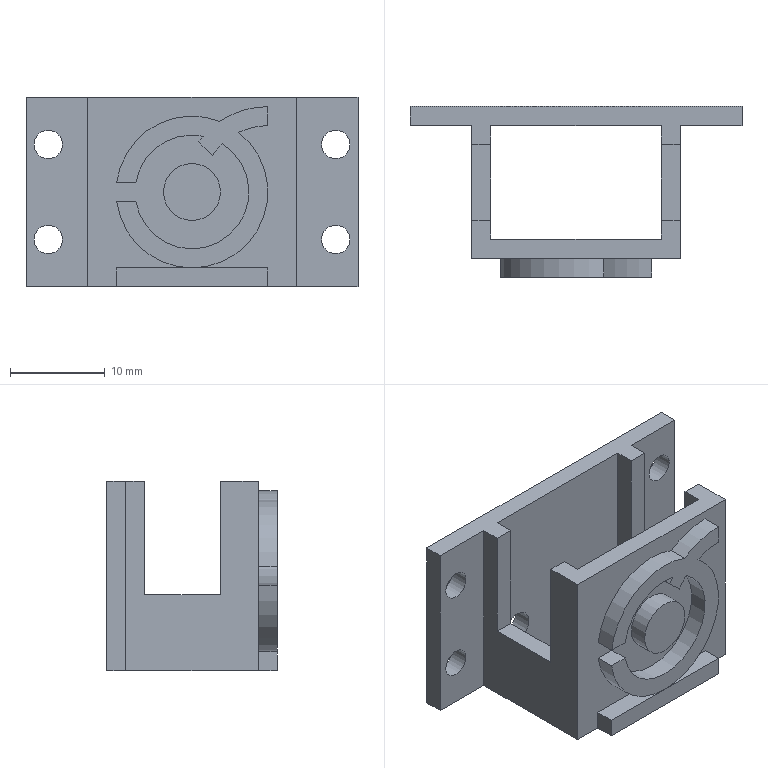Part | NX | features BREP 4 | 4 solids | 50 faces | box 35 x 18 x 20 mm | volume 3071 mm3 | plane 35 | cylinder 15 | commonest cylinder face diameters 3 x4 3.5 x2 12 x2 14 x2 16 x2 18 x2
STEP:
#1=CARTESIAN_POINT('',(-8.,-8.,-10.));
#2=VERTEX_POINT('',#1);
#3=CARTESIAN_POINT('',(-8.,-8.,-8.));
#4=VERTEX_POINT('',#3);
#5=CARTESIAN_POINT('',(-8.,-8.,-8.));
#6=DIRECTION('',(0.,0.,1.));
#7=VECTOR('',#6,1000.);
#8=LINE('',#5,#7);
#9=EDGE_CURVE('',#2,#4,#8,.T.);
#10=ORIENTED_EDGE('',*,*,#9,.F.);
#11=CARTESIAN_POINT('',(-8.,-10.,-10.));
#12=VERTEX_POINT('',#11);
#13=CARTESIAN_POINT('',(-8.,8.125,-10.));
#14=DIRECTION('',(0.,-1.,0.));
#15=VECTOR('',#14,1000.);
#16=LINE('',#13,#15);
#17=EDGE_CURVE('',#2,#12,#16,.T.);
#18=ORIENTED_EDGE('',*,*,#17,.T.);
#19=CARTESIAN_POINT('',(-8.,-10.,-8.));
#20=VERTEX_POINT('',#19);
#21=CARTESIAN_POINT('',(-8.,-10.,-8.));
#22=DIRECTION('',(0.,0.,-1.));
#23=VECTOR('',#22,1000.);
#24=LINE('',#21,#23);
#25=EDGE_CURVE('',#20,#12,#24,.T.);
#26=ORIENTED_EDGE('',*,*,#25,.F.);
#27=CARTESIAN_POINT('',(-8.,8.125,-8.));
#28=DIRECTION('',(0.,-1.,0.));
#29=VECTOR('',#28,1000.);
#30=LINE('',#27,#29);
#31=EDGE_CURVE('',#4,#20,#30,.T.);
#32=ORIENTED_EDGE('',*,*,#31,.F.);
#33=EDGE_LOOP('',(#10,#18,#26,#32));
#34=FACE_BOUND('',#33,.T.);
#35=CARTESIAN_POINT('',(-8.,8.125,-8.));
#36=DIRECTION('',(-1.,0.,0.));
#37=DIRECTION('',(0.,0.,1.));
#38=AXIS2_PLACEMENT_3D('',#35,#36,#37);
#39=PLANE('',#38);
#40=ADVANCED_FACE('',(#34),#39,.T.);
#41=CARTESIAN_POINT('',(8.,-8.,-8.));
#42=VERTEX_POINT('',#41);
#43=CARTESIAN_POINT('',(-8.,-8.,-8.));
#44=DIRECTION('',(1.,0.,0.));
#45=VECTOR('',#44,1000.);
#46=LINE('',#43,#45);
#47=EDGE_CURVE('',#4,#42,#46,.T.);
#48=ORIENTED_EDGE('',*,*,#47,.F.);
#49=ORIENTED_EDGE('',*,*,#31,.T.);
#50=CARTESIAN_POINT('',(8.,-10.,-8.));
#51=VERTEX_POINT('',#50);
#52=CARTESIAN_POINT('',(-8.,-10.,-8.));
#53=DIRECTION('',(-1.,0.,0.));
#54=VECTOR('',#53,1000.);
#55=LINE('',#52,#54);
#56=EDGE_CURVE('',#51,#20,#55,.T.);
#57=ORIENTED_EDGE('',*,*,#56,.F.);
#58=CARTESIAN_POINT('',(8.,8.125,-8.));
#59=DIRECTION('',(0.,-1.,0.));
#60=VECTOR('',#59,1000.);
#61=LINE('',#58,#60);
#62=EDGE_CURVE('',#42,#51,#61,.T.);
#63=ORIENTED_EDGE('',*,*,#62,.F.);
#64=EDGE_LOOP('',(#48,#49,#57,#63));
#65=FACE_BOUND('',#64,.T.);
#66=CARTESIAN_POINT('',(-8.,8.125,-8.));
#67=DIRECTION('',(0.,0.,1.));
#68=DIRECTION('',(1.,0.,0.));
#69=AXIS2_PLACEMENT_3D('',#66,#67,#68);
#70=PLANE('',#69);
#71=ADVANCED_FACE('',(#65),#70,.T.);
#72=CARTESIAN_POINT('',(8.,-8.,-10.));
#73=VERTEX_POINT('',#72);
#74=CARTESIAN_POINT('',(8.,-8.,-8.));
#75=DIRECTION('',(0.,0.,-1.));
#76=VECTOR('',#75,1000.);
#77=LINE('',#74,#76);
#78=EDGE_CURVE('',#42,#73,#77,.T.);
#79=ORIENTED_EDGE('',*,*,#78,.F.);
#80=ORIENTED_EDGE('',*,*,#62,.T.);
#81=CARTESIAN_POINT('',(8.,-10.,-10.));
#82=VERTEX_POINT('',#81);
#83=CARTESIAN_POINT('',(8.,-10.,-8.));
#84=DIRECTION('',(0.,0.,1.));
#85=VECTOR('',#84,1000.);
#86=LINE('',#83,#85);
#87=EDGE_CURVE('',#82,#51,#86,.T.);
#88=ORIENTED_EDGE('',*,*,#87,.F.);
#89=CARTESIAN_POINT('',(8.,8.125,-10.));
#90=DIRECTION('',(0.,-1.,0.));
#91=VECTOR('',#90,1000.);
#92=LINE('',#89,#91);
#93=EDGE_CURVE('',#73,#82,#92,.T.);
#94=ORIENTED_EDGE('',*,*,#93,.F.);
#95=EDGE_LOOP('',(#79,#80,#88,#94));
#96=FACE_BOUND('',#95,.T.);
#97=CARTESIAN_POINT('',(8.,8.125,-8.));
#98=DIRECTION('',(1.,0.,0.));
#99=DIRECTION('',(0.,-1.,0.));
#100=AXIS2_PLACEMENT_3D('',#97,#98,#99);
#101=PLANE('',#100);
#102=ADVANCED_FACE('',(#96),#101,.T.);
#103=CARTESIAN_POINT('',(-8.,-8.,-10.));
#104=DIRECTION('',(-1.,0.,0.));
#105=VECTOR('',#104,1000.);
#106=LINE('',#103,#105);
#107=EDGE_CURVE('',#73,#2,#106,.T.);
#108=ORIENTED_EDGE('',*,*,#107,.F.);
#109=ORIENTED_EDGE('',*,*,#93,.T.);
#110=CARTESIAN_POINT('',(-8.,-10.,-10.));
#111=DIRECTION('',(1.,0.,0.));
#112=VECTOR('',#111,1000.);
#113=LINE('',#110,#112);
#114=EDGE_CURVE('',#12,#82,#113,.T.);
#115=ORIENTED_EDGE('',*,*,#114,.F.);
#116=ORIENTED_EDGE('',*,*,#17,.F.);
#117=EDGE_LOOP('',(#108,#109,#115,#116));
#118=FACE_BOUND('',#117,.T.);
#119=CARTESIAN_POINT('',(-8.,8.125,-10.));
#120=DIRECTION('',(0.,0.,-1.));
#121=DIRECTION('',(-1.,0.,0.));
#122=AXIS2_PLACEMENT_3D('',#119,#120,#121);
#123=PLANE('',#122);
#124=ADVANCED_FACE('',(#118),#123,.T.);
#125=ORIENTED_EDGE('',*,*,#25,.T.);
#126=ORIENTED_EDGE('',*,*,#114,.T.);
#127=ORIENTED_EDGE('',*,*,#87,.T.);
#128=ORIENTED_EDGE('',*,*,#56,.T.);
#129=EDGE_LOOP('',(#125,#126,#127,#128));
#130=FACE_BOUND('',#129,.T.);
#131=CARTESIAN_POINT('',(0.,-10.,0.));
#132=DIRECTION('',(0.,-1.,0.));
#133=DIRECTION('',(-1.,0.,0.));
#134=AXIS2_PLACEMENT_3D('',#131,#132,#133);
#135=PLANE('',#134);
#136=ADVANCED_FACE('',(#130),#135,.T.);
#137=ORIENTED_EDGE('',*,*,#9,.T.);
#138=ORIENTED_EDGE('',*,*,#47,.T.);
#139=ORIENTED_EDGE('',*,*,#78,.T.);
#140=ORIENTED_EDGE('',*,*,#107,.T.);
#141=EDGE_LOOP('',(#137,#138,#139,#140));
#142=FACE_BOUND('',#141,.T.);
#143=CARTESIAN_POINT('',(0.,-8.,0.));
#144=DIRECTION('',(0.,-1.,0.));
#145=DIRECTION('',(-1.,0.,0.));
#146=AXIS2_PLACEMENT_3D('',#143,#144,#145);
#147=PLANE('',#146);
#148=ADVANCED_FACE('',(#142),#147,.F.);
#149=CLOSED_SHELL('',(#40,#71,#102,#124,#136,#148));
#150=MANIFOLD_SOLID_BREP('',#149);
#151=CARTESIAN_POINT('',(3.,-10.,0.));
#152=VERTEX_POINT('',#151);
#153=CARTESIAN_POINT('',(0.,-10.,0.));
#154=DIRECTION('',(0.,-1.,0.));
#155=DIRECTION('',(1.,0.,0.));
#156=AXIS2_PLACEMENT_3D('',#153,#154,#155);
#157=CIRCLE('',#156,3.);
#158=EDGE_CURVE('',#152,#152,#157,.T.);
#159=ORIENTED_EDGE('',*,*,#158,.F.);
#160=EDGE_LOOP('',(#159));
#161=FACE_BOUND('',#160,.T.);
#162=CARTESIAN_POINT('',(3.,-8.,0.));
#163=VERTEX_POINT('',#162);
#164=CARTESIAN_POINT('',(0.,-8.,0.));
#165=DIRECTION('',(0.,1.,0.));
#166=DIRECTION('',(1.,0.,0.));
#167=AXIS2_PLACEMENT_3D('',#164,#165,#166);
#168=CIRCLE('',#167,3.);
#169=EDGE_CURVE('',#163,#163,#168,.T.);
#170=ORIENTED_EDGE('',*,*,#169,.F.);
#171=EDGE_LOOP('',(#170));
#172=FACE_BOUND('',#171,.T.);
#173=CARTESIAN_POINT('',(0.,0.4853,0.));
#174=DIRECTION('',(0.,-1.,0.));
#175=DIRECTION('',(-1.,0.,0.));
#176=AXIS2_PLACEMENT_3D('',#173,#174,#175);
#177=CYLINDRICAL_SURFACE('',#176,3.);
#178=ADVANCED_FACE('',(#161,#172),#177,.T.);
#179=ORIENTED_EDGE('',*,*,#158,.T.);
#180=EDGE_LOOP('',(#179));
#181=FACE_BOUND('',#180,.T.);
#182=CARTESIAN_POINT('',(0.,-10.,0.));
#183=DIRECTION('',(0.,-1.,0.));
#184=DIRECTION('',(-1.,0.,0.));
#185=AXIS2_PLACEMENT_3D('',#182,#183,#184);
#186=PLANE('',#185);
#187=ADVANCED_FACE('',(#181),#186,.T.);
#188=ORIENTED_EDGE('',*,*,#169,.T.);
#189=EDGE_LOOP('',(#188));
#190=FACE_BOUND('',#189,.T.);
#191=CARTESIAN_POINT('',(0.,-8.,0.));
#192=DIRECTION('',(0.,-1.,0.));
#193=DIRECTION('',(-1.,0.,0.));
#194=AXIS2_PLACEMENT_3D('',#191,#192,#193);
#195=PLANE('',#194);
#196=ADVANCED_FACE('',(#190),#195,.F.);
#197=CLOSED_SHELL('',(#178,#187,#196));
#198=MANIFOLD_SOLID_BREP('',#197);
#199=CARTESIAN_POINT('',(2.938,-8.,7.441));
#200=VERTEX_POINT('',#199);
#201=CARTESIAN_POINT('',(-7.937,-8.,1.));
#202=VERTEX_POINT('',#201);
#203=CARTESIAN_POINT('',(0.,-8.,0.));
#204=DIRECTION('',(0.,-1.,0.));
#205=DIRECTION('',(1.,0.,0.));
#206=AXIS2_PLACEMENT_3D('',#203,#204,#205);
#207=CIRCLE('',#206,8.);
#208=EDGE_CURVE('',#200,#202,#207,.T.);
#209=ORIENTED_EDGE('',*,*,#208,.T.);
#210=CARTESIAN_POINT('',(-7.937,-10.,1.));
#211=VERTEX_POINT('',#210);
#212=CARTESIAN_POINT('',(-7.937,-10.,1.));
#213=DIRECTION('',(0.,-1.,0.));
#214=VECTOR('',#213,1000.);
#215=LINE('',#212,#214);
#216=EDGE_CURVE('',#202,#211,#215,.T.);
#217=ORIENTED_EDGE('',*,*,#216,.T.);
#218=CARTESIAN_POINT('',(2.938,-10.,7.441));
#219=VERTEX_POINT('',#218);
#220=CARTESIAN_POINT('',(0.,-10.,0.));
#221=DIRECTION('',(0.,-1.,0.));
#222=DIRECTION('',(1.,0.,0.));
#223=AXIS2_PLACEMENT_3D('',#220,#221,#222);
#224=CIRCLE('',#223,8.);
#225=EDGE_CURVE('',#219,#211,#224,.T.);
#226=ORIENTED_EDGE('',*,*,#225,.F.);
#227=CARTESIAN_POINT('',(2.938,-9.,7.441));
#228=DIRECTION('',(0.,1.,0.));
#229=VECTOR('',#228,1000.);
#230=LINE('',#227,#229);
#231=EDGE_CURVE('',#219,#200,#230,.T.);
#232=ORIENTED_EDGE('',*,*,#231,.T.);
#233=EDGE_LOOP('',(#209,#217,#226,#232));
#234=FACE_BOUND('',#233,.T.);
#235=CARTESIAN_POINT('',(0.,-10.,0.));
#236=DIRECTION('',(0.,1.,0.));
#237=DIRECTION('',(1.,0.,0.));
#238=AXIS2_PLACEMENT_3D('',#235,#236,#237);
#239=CYLINDRICAL_SURFACE('',#238,8.);
#240=ADVANCED_FACE('',(#234),#239,.T.);
#241=CARTESIAN_POINT('',(-5.916,-8.,1.));
#242=VERTEX_POINT('',#241);
#243=CARTESIAN_POINT('',(-5.916,-10.,1.));
#244=VERTEX_POINT('',#243);
#245=CARTESIAN_POINT('',(-5.916,-10.,1.));
#246=DIRECTION('',(0.,-1.,0.));
#247=VECTOR('',#246,1000.);
#248=LINE('',#245,#247);
#249=EDGE_CURVE('',#242,#244,#248,.T.);
#250=ORIENTED_EDGE('',*,*,#249,.F.);
#251=CARTESIAN_POINT('',(1.188,-8.,5.881));
#252=VERTEX_POINT('',#251);
#253=CARTESIAN_POINT('',(0.,-8.,0.));
#254=DIRECTION('',(0.,-1.,0.));
#255=DIRECTION('',(1.,0.,0.));
#256=AXIS2_PLACEMENT_3D('',#253,#254,#255);
#257=CIRCLE('',#256,6.);
#258=EDGE_CURVE('',#252,#242,#257,.T.);
#259=ORIENTED_EDGE('',*,*,#258,.F.);
#260=CARTESIAN_POINT('',(1.188,-10.,5.881));
#261=VERTEX_POINT('',#260);
#262=CARTESIAN_POINT('',(1.188,-9.,5.881));
#263=DIRECTION('',(0.,1.,0.));
#264=VECTOR('',#263,1000.);
#265=LINE('',#262,#264);
#266=EDGE_CURVE('',#261,#252,#265,.T.);
#267=ORIENTED_EDGE('',*,*,#266,.F.);
#268=CARTESIAN_POINT('',(0.,-10.,0.));
#269=DIRECTION('',(0.,-1.,0.));
#270=DIRECTION('',(1.,0.,0.));
#271=AXIS2_PLACEMENT_3D('',#268,#269,#270);
#272=CIRCLE('',#271,6.);
#273=EDGE_CURVE('',#261,#244,#272,.T.);
#274=ORIENTED_EDGE('',*,*,#273,.T.);
#275=EDGE_LOOP('',(#250,#259,#267,#274));
#276=FACE_BOUND('',#275,.T.);
#277=CARTESIAN_POINT('',(0.,-10.,0.));
#278=DIRECTION('',(0.,1.,0.));
#279=DIRECTION('',(1.,0.,0.));
#280=AXIS2_PLACEMENT_3D('',#277,#278,#279);
#281=CYLINDRICAL_SURFACE('',#280,6.);
#282=ADVANCED_FACE('',(#276),#281,.F.);
#283=CARTESIAN_POINT('',(-10.409,-10.,1.));
#284=DIRECTION('',(-1.,0.,0.));
#285=VECTOR('',#284,1000.);
#286=LINE('',#283,#285);
#287=EDGE_CURVE('',#244,#211,#286,.T.);
#288=ORIENTED_EDGE('',*,*,#287,.F.);
#289=ORIENTED_EDGE('',*,*,#273,.F.);
#290=CARTESIAN_POINT('',(0.7151,-10.,5.285));
#291=VERTEX_POINT('',#290);
#292=CARTESIAN_POINT('',(8.,-10.,0.));
#293=DIRECTION('',(0.,-1.,0.));
#294=DIRECTION('',(1.,0.,0.));
#295=AXIS2_PLACEMENT_3D('',#292,#293,#294);
#296=CIRCLE('',#295,9.);
#297=EDGE_CURVE('',#261,#291,#296,.T.);
#298=ORIENTED_EDGE('',*,*,#297,.T.);
#299=CARTESIAN_POINT('',(2.152,-10.,3.848));
#300=VERTEX_POINT('',#299);
#301=CARTESIAN_POINT('',(2.152,-10.,3.848));
#302=DIRECTION('',(0.7071,0.,-0.7071));
#303=VECTOR('',#302,1000.);
#304=LINE('',#301,#303);
#305=EDGE_CURVE('',#291,#300,#304,.T.);
#306=ORIENTED_EDGE('',*,*,#305,.T.);
#307=CARTESIAN_POINT('',(3.188,-10.,5.083));
#308=VERTEX_POINT('',#307);
#309=CARTESIAN_POINT('',(8.,-10.,0.));
#310=DIRECTION('',(0.,1.,0.));
#311=DIRECTION('',(1.,0.,0.));
#312=AXIS2_PLACEMENT_3D('',#309,#310,#311);
#313=CIRCLE('',#312,7.);
#314=EDGE_CURVE('',#300,#308,#313,.T.);
#315=ORIENTED_EDGE('',*,*,#314,.T.);
#316=CARTESIAN_POINT('',(-5.916,-10.,-1.));
#317=VERTEX_POINT('',#316);
#318=CARTESIAN_POINT('',(0.,-10.,0.));
#319=DIRECTION('',(0.,-1.,0.));
#320=DIRECTION('',(1.,0.,0.));
#321=AXIS2_PLACEMENT_3D('',#318,#319,#320);
#322=CIRCLE('',#321,6.);
#323=EDGE_CURVE('',#317,#308,#322,.T.);
#324=ORIENTED_EDGE('',*,*,#323,.F.);
#325=CARTESIAN_POINT('',(-7.937,-10.,-1.));
#326=VERTEX_POINT('',#325);
#327=CARTESIAN_POINT('',(-10.409,-10.,-1.));
#328=DIRECTION('',(1.,0.,0.));
#329=VECTOR('',#328,1000.);
#330=LINE('',#327,#329);
#331=EDGE_CURVE('',#326,#317,#330,.T.);
#332=ORIENTED_EDGE('',*,*,#331,.F.);
#333=CARTESIAN_POINT('',(4.938,-10.,6.295));
#334=VERTEX_POINT('',#333);
#335=CARTESIAN_POINT('',(0.,-10.,0.));
#336=DIRECTION('',(0.,-1.,0.));
#337=DIRECTION('',(1.,0.,0.));
#338=AXIS2_PLACEMENT_3D('',#335,#336,#337);
#339=CIRCLE('',#338,8.);
#340=EDGE_CURVE('',#326,#334,#339,.T.);
#341=ORIENTED_EDGE('',*,*,#340,.T.);
#342=CARTESIAN_POINT('',(8.,-10.,7.));
#343=VERTEX_POINT('',#342);
#344=CARTESIAN_POINT('',(8.,-10.,0.));
#345=DIRECTION('',(0.,1.,0.));
#346=DIRECTION('',(1.,0.,0.));
#347=AXIS2_PLACEMENT_3D('',#344,#345,#346);
#348=CIRCLE('',#347,7.);
#349=EDGE_CURVE('',#334,#343,#348,.T.);
#350=ORIENTED_EDGE('',*,*,#349,.T.);
#351=CARTESIAN_POINT('',(8.,-10.,9.));
#352=VERTEX_POINT('',#351);
#353=CARTESIAN_POINT('',(8.,-10.,7.));
#354=DIRECTION('',(0.,0.,1.));
#355=VECTOR('',#354,1000.);
#356=LINE('',#353,#355);
#357=EDGE_CURVE('',#343,#352,#356,.T.);
#358=ORIENTED_EDGE('',*,*,#357,.T.);
#359=CARTESIAN_POINT('',(8.,-10.,0.));
#360=DIRECTION('',(0.,-1.,0.));
#361=DIRECTION('',(1.,0.,0.));
#362=AXIS2_PLACEMENT_3D('',#359,#360,#361);
#363=CIRCLE('',#362,9.);
#364=EDGE_CURVE('',#352,#219,#363,.T.);
#365=ORIENTED_EDGE('',*,*,#364,.T.);
#366=ORIENTED_EDGE('',*,*,#225,.T.);
#367=EDGE_LOOP('',(#288,#289,#298,#306,#315,#324,#332,#341,#350,#358,#365,#366));
#368=FACE_BOUND('',#367,.T.);
#369=CARTESIAN_POINT('',(0.,-10.,0.));
#370=DIRECTION('',(0.,-1.,0.));
#371=DIRECTION('',(-1.,0.,0.));
#372=AXIS2_PLACEMENT_3D('',#369,#370,#371);
#373=PLANE('',#372);
#374=ADVANCED_FACE('',(#368),#373,.T.);
#375=ORIENTED_EDGE('',*,*,#258,.T.);
#376=CARTESIAN_POINT('',(-10.409,-8.,1.));
#377=DIRECTION('',(-1.,0.,0.));
#378=VECTOR('',#377,1000.);
#379=LINE('',#376,#378);
#380=EDGE_CURVE('',#242,#202,#379,.T.);
#381=ORIENTED_EDGE('',*,*,#380,.T.);
#382=ORIENTED_EDGE('',*,*,#208,.F.);
#383=CARTESIAN_POINT('',(8.,-8.,9.));
#384=VERTEX_POINT('',#383);
#385=CARTESIAN_POINT('',(8.,-8.,0.));
#386=DIRECTION('',(0.,1.,0.));
#387=DIRECTION('',(1.,0.,0.));
#388=AXIS2_PLACEMENT_3D('',#385,#386,#387);
#389=CIRCLE('',#388,9.);
#390=EDGE_CURVE('',#200,#384,#389,.T.);
#391=ORIENTED_EDGE('',*,*,#390,.T.);
#392=CARTESIAN_POINT('',(8.,-8.,7.));
#393=VERTEX_POINT('',#392);
#394=CARTESIAN_POINT('',(8.,-8.,7.));
#395=DIRECTION('',(0.,0.,-1.));
#396=VECTOR('',#395,1000.);
#397=LINE('',#394,#396);
#398=EDGE_CURVE('',#384,#393,#397,.T.);
#399=ORIENTED_EDGE('',*,*,#398,.T.);
#400=CARTESIAN_POINT('',(4.938,-8.,6.295));
#401=VERTEX_POINT('',#400);
#402=CARTESIAN_POINT('',(8.,-8.,0.));
#403=DIRECTION('',(0.,-1.,0.));
#404=DIRECTION('',(1.,0.,0.));
#405=AXIS2_PLACEMENT_3D('',#402,#403,#404);
#406=CIRCLE('',#405,7.);
#407=EDGE_CURVE('',#393,#401,#406,.T.);
#408=ORIENTED_EDGE('',*,*,#407,.T.);
#409=CARTESIAN_POINT('',(-7.937,-8.,-1.));
#410=VERTEX_POINT('',#409);
#411=CARTESIAN_POINT('',(0.,-8.,0.));
#412=DIRECTION('',(0.,-1.,0.));
#413=DIRECTION('',(1.,0.,0.));
#414=AXIS2_PLACEMENT_3D('',#411,#412,#413);
#415=CIRCLE('',#414,8.);
#416=EDGE_CURVE('',#410,#401,#415,.T.);
#417=ORIENTED_EDGE('',*,*,#416,.F.);
#418=CARTESIAN_POINT('',(-5.916,-8.,-1.));
#419=VERTEX_POINT('',#418);
#420=CARTESIAN_POINT('',(-10.409,-8.,-1.));
#421=DIRECTION('',(1.,0.,0.));
#422=VECTOR('',#421,1000.);
#423=LINE('',#420,#422);
#424=EDGE_CURVE('',#410,#419,#423,.T.);
#425=ORIENTED_EDGE('',*,*,#424,.T.);
#426=CARTESIAN_POINT('',(3.188,-8.,5.083));
#427=VERTEX_POINT('',#426);
#428=CARTESIAN_POINT('',(0.,-8.,0.));
#429=DIRECTION('',(0.,-1.,0.));
#430=DIRECTION('',(1.,0.,0.));
#431=AXIS2_PLACEMENT_3D('',#428,#429,#430);
#432=CIRCLE('',#431,6.);
#433=EDGE_CURVE('',#419,#427,#432,.T.);
#434=ORIENTED_EDGE('',*,*,#433,.T.);
#435=CARTESIAN_POINT('',(2.152,-8.,3.848));
#436=VERTEX_POINT('',#435);
#437=CARTESIAN_POINT('',(8.,-8.,0.));
#438=DIRECTION('',(0.,-1.,0.));
#439=DIRECTION('',(1.,0.,0.));
#440=AXIS2_PLACEMENT_3D('',#437,#438,#439);
#441=CIRCLE('',#440,7.);
#442=EDGE_CURVE('',#427,#436,#441,.T.);
#443=ORIENTED_EDGE('',*,*,#442,.T.);
#444=CARTESIAN_POINT('',(0.7151,-8.,5.285));
#445=VERTEX_POINT('',#444);
#446=CARTESIAN_POINT('',(2.152,-8.,3.848));
#447=DIRECTION('',(-0.7071,0.,0.7071));
#448=VECTOR('',#447,1000.);
#449=LINE('',#446,#448);
#450=EDGE_CURVE('',#436,#445,#449,.T.);
#451=ORIENTED_EDGE('',*,*,#450,.T.);
#452=CARTESIAN_POINT('',(8.,-8.,0.));
#453=DIRECTION('',(0.,1.,0.));
#454=DIRECTION('',(1.,0.,0.));
#455=AXIS2_PLACEMENT_3D('',#452,#453,#454);
#456=CIRCLE('',#455,9.);
#457=EDGE_CURVE('',#445,#252,#456,.T.);
#458=ORIENTED_EDGE('',*,*,#457,.T.);
#459=EDGE_LOOP('',(#375,#381,#382,#391,#399,#408,#417,#425,#434,#443,#451,#458));
#460=FACE_BOUND('',#459,.T.);
#461=CARTESIAN_POINT('',(0.,-8.,0.));
#462=DIRECTION('',(0.,-1.,0.));
#463=DIRECTION('',(-1.,0.,0.));
#464=AXIS2_PLACEMENT_3D('',#461,#462,#463);
#465=PLANE('',#464);
#466=ADVANCED_FACE('',(#460),#465,.F.);
#467=ORIENTED_EDGE('',*,*,#340,.F.);
#468=CARTESIAN_POINT('',(-7.937,-10.,-1.));
#469=DIRECTION('',(0.,1.,0.));
#470=VECTOR('',#469,1000.);
#471=LINE('',#468,#470);
#472=EDGE_CURVE('',#326,#410,#471,.T.);
#473=ORIENTED_EDGE('',*,*,#472,.T.);
#474=ORIENTED_EDGE('',*,*,#416,.T.);
#475=CARTESIAN_POINT('',(4.938,-9.,6.295));
#476=DIRECTION('',(0.,-1.,0.));
#477=VECTOR('',#476,1000.);
#478=LINE('',#475,#477);
#479=EDGE_CURVE('',#401,#334,#478,.T.);
#480=ORIENTED_EDGE('',*,*,#479,.T.);
#481=EDGE_LOOP('',(#467,#473,#474,#480));
#482=FACE_BOUND('',#481,.T.);
#483=CARTESIAN_POINT('',(0.,-10.,0.));
#484=DIRECTION('',(0.,1.,0.));
#485=DIRECTION('',(1.,0.,0.));
#486=AXIS2_PLACEMENT_3D('',#483,#484,#485);
#487=CYLINDRICAL_SURFACE('',#486,8.);
#488=ADVANCED_FACE('',(#482),#487,.T.);
#489=CARTESIAN_POINT('',(-5.916,-10.,-1.));
#490=DIRECTION('',(0.,1.,0.));
#491=VECTOR('',#490,1000.);
#492=LINE('',#489,#491);
#493=EDGE_CURVE('',#317,#419,#492,.T.);
#494=ORIENTED_EDGE('',*,*,#493,.F.);
#495=ORIENTED_EDGE('',*,*,#323,.T.);
#496=CARTESIAN_POINT('',(3.188,-9.,5.083));
#497=DIRECTION('',(0.,-1.,0.));
#498=VECTOR('',#497,1000.);
#499=LINE('',#496,#498);
#500=EDGE_CURVE('',#427,#308,#499,.T.);
#501=ORIENTED_EDGE('',*,*,#500,.F.);
#502=ORIENTED_EDGE('',*,*,#433,.F.);
#503=EDGE_LOOP('',(#494,#495,#501,#502));
#504=FACE_BOUND('',#503,.T.);
#505=CARTESIAN_POINT('',(0.,-10.,0.));
#506=DIRECTION('',(0.,1.,0.));
#507=DIRECTION('',(1.,0.,0.));
#508=AXIS2_PLACEMENT_3D('',#505,#506,#507);
#509=CYLINDRICAL_SURFACE('',#508,6.);
#510=ADVANCED_FACE('',(#504),#509,.F.);
#511=ORIENTED_EDGE('',*,*,#450,.F.);
#512=CARTESIAN_POINT('',(2.152,0.9228,3.848));
#513=DIRECTION('',(0.,-1.,0.));
#514=VECTOR('',#513,1000.);
#515=LINE('',#512,#514);
#516=EDGE_CURVE('',#436,#300,#515,.T.);
#517=ORIENTED_EDGE('',*,*,#516,.T.);
#518=ORIENTED_EDGE('',*,*,#305,.F.);
#519=CARTESIAN_POINT('',(0.7151,0.9228,5.285));
#520=DIRECTION('',(0.,-1.,0.));
#521=VECTOR('',#520,1000.);
#522=LINE('',#519,#521);
#523=EDGE_CURVE('',#445,#291,#522,.T.);
#524=ORIENTED_EDGE('',*,*,#523,.F.);
#525=EDGE_LOOP('',(#511,#517,#518,#524));
#526=FACE_BOUND('',#525,.T.);
#527=CARTESIAN_POINT('',(2.152,0.9228,3.848));
#528=DIRECTION('',(-0.7071,0.,-0.7071));
#529=DIRECTION('',(-0.7071,0.,0.7071));
#530=AXIS2_PLACEMENT_3D('',#527,#528,#529);
#531=PLANE('',#530);
#532=ADVANCED_FACE('',(#526),#531,.T.);
#533=ORIENTED_EDGE('',*,*,#297,.F.);
#534=ORIENTED_EDGE('',*,*,#266,.T.);
#535=ORIENTED_EDGE('',*,*,#457,.F.);
#536=ORIENTED_EDGE('',*,*,#523,.T.);
#537=EDGE_LOOP('',(#533,#534,#535,#536));
#538=FACE_BOUND('',#537,.T.);
#539=CARTESIAN_POINT('',(8.,0.9228,0.));
#540=DIRECTION('',(0.,-1.,0.));
#541=DIRECTION('',(-1.,0.,0.));
#542=AXIS2_PLACEMENT_3D('',#539,#540,#541);
#543=CYLINDRICAL_SURFACE('',#542,9.);
#544=ADVANCED_FACE('',(#538),#543,.T.);
#545=ORIENTED_EDGE('',*,*,#442,.F.);
#546=ORIENTED_EDGE('',*,*,#500,.T.);
#547=ORIENTED_EDGE('',*,*,#314,.F.);
#548=ORIENTED_EDGE('',*,*,#516,.F.);
#549=EDGE_LOOP('',(#545,#546,#547,#548));
#550=FACE_BOUND('',#549,.T.);
#551=CARTESIAN_POINT('',(8.,0.9228,0.));
#552=DIRECTION('',(0.,-1.,0.));
#553=DIRECTION('',(-1.,0.,0.));
#554=AXIS2_PLACEMENT_3D('',#551,#552,#553);
#555=CYLINDRICAL_SURFACE('',#554,7.);
#556=ADVANCED_FACE('',(#550),#555,.F.);
#557=ORIENTED_EDGE('',*,*,#479,.F.);
#558=ORIENTED_EDGE('',*,*,#407,.F.);
#559=CARTESIAN_POINT('',(8.,0.9228,7.));
#560=DIRECTION('',(0.,-1.,0.));
#561=VECTOR('',#560,1000.);
#562=LINE('',#559,#561);
#563=EDGE_CURVE('',#393,#343,#562,.T.);
#564=ORIENTED_EDGE('',*,*,#563,.T.);
#565=ORIENTED_EDGE('',*,*,#349,.F.);
#566=EDGE_LOOP('',(#557,#558,#564,#565));
#567=FACE_BOUND('',#566,.T.);
#568=CARTESIAN_POINT('',(8.,0.9228,0.));
#569=DIRECTION('',(0.,-1.,0.));
#570=DIRECTION('',(-1.,0.,0.));
#571=AXIS2_PLACEMENT_3D('',#568,#569,#570);
#572=CYLINDRICAL_SURFACE('',#571,7.);
#573=ADVANCED_FACE('',(#567),#572,.F.);
#574=ORIENTED_EDGE('',*,*,#231,.F.);
#575=ORIENTED_EDGE('',*,*,#364,.F.);
#576=CARTESIAN_POINT('',(8.,0.9228,9.));
#577=DIRECTION('',(0.,-1.,0.));
#578=VECTOR('',#577,1000.);
#579=LINE('',#576,#578);
#580=EDGE_CURVE('',#384,#352,#579,.T.);
#581=ORIENTED_EDGE('',*,*,#580,.F.);
#582=ORIENTED_EDGE('',*,*,#390,.F.);
#583=EDGE_LOOP('',(#574,#575,#581,#582));
#584=FACE_BOUND('',#583,.T.);
#585=CARTESIAN_POINT('',(8.,0.9228,0.));
#586=DIRECTION('',(0.,-1.,0.));
#587=DIRECTION('',(-1.,0.,0.));
#588=AXIS2_PLACEMENT_3D('',#585,#586,#587);
#589=CYLINDRICAL_SURFACE('',#588,9.);
#590=ADVANCED_FACE('',(#584),#589,.T.);
#591=ORIENTED_EDGE('',*,*,#398,.F.);
#592=ORIENTED_EDGE('',*,*,#580,.T.);
#593=ORIENTED_EDGE('',*,*,#357,.F.);
#594=ORIENTED_EDGE('',*,*,#563,.F.);
#595=EDGE_LOOP('',(#591,#592,#593,#594));
#596=FACE_BOUND('',#595,.T.);
#597=CARTESIAN_POINT('',(8.,0.9228,7.));
#598=DIRECTION('',(1.,0.,0.));
#599=DIRECTION('',(0.,-1.,0.));
#600=AXIS2_PLACEMENT_3D('',#597,#598,#599);
#601=PLANE('',#600);
#602=ADVANCED_FACE('',(#596),#601,.T.);
#603=ORIENTED_EDGE('',*,*,#331,.T.);
#604=ORIENTED_EDGE('',*,*,#493,.T.);
#605=ORIENTED_EDGE('',*,*,#424,.F.);
#606=ORIENTED_EDGE('',*,*,#472,.F.);
#607=EDGE_LOOP('',(#603,#604,#605,#606));
#608=FACE_BOUND('',#607,.T.);
#609=CARTESIAN_POINT('',(-10.409,-8.,-1.));
#610=DIRECTION('',(0.,0.,-1.));
#611=DIRECTION('',(-1.,0.,0.));
#612=AXIS2_PLACEMENT_3D('',#609,#610,#611);
#613=PLANE('',#612);
#614=ADVANCED_FACE('',(#608),#613,.F.);
#615=ORIENTED_EDGE('',*,*,#380,.F.);
#616=ORIENTED_EDGE('',*,*,#249,.T.);
#617=ORIENTED_EDGE('',*,*,#287,.T.);
#618=ORIENTED_EDGE('',*,*,#216,.F.);
#619=EDGE_LOOP('',(#615,#616,#617,#618));
#620=FACE_BOUND('',#619,.T.);
#621=CARTESIAN_POINT('',(-10.409,-8.,1.));
#622=DIRECTION('',(0.,0.,1.));
#623=DIRECTION('',(1.,0.,0.));
#624=AXIS2_PLACEMENT_3D('',#621,#622,#623);
#625=PLANE('',#624);
#626=ADVANCED_FACE('',(#620),#625,.F.);
#627=CLOSED_SHELL('',(#240,#282,#374,#466,#488,#510,#532,#544,#556,#573,#590,#602,#614,#626));
#628=MANIFOLD_SOLID_BREP('',#627);
#629=CARTESIAN_POINT('',(15.15,6.,-3.5));
#630=VERTEX_POINT('',#629);
#631=CARTESIAN_POINT('',(15.15,6.,-5.));
#632=DIRECTION('',(0.,-1.,0.));
#633=DIRECTION('',(0.,0.,1.));
#634=AXIS2_PLACEMENT_3D('',#631,#632,#633);
#635=CIRCLE('',#634,1.5);
#636=EDGE_CURVE('',#630,#630,#635,.T.);
#637=ORIENTED_EDGE('',*,*,#636,.T.);
#638=EDGE_LOOP('',(#637));
#639=FACE_BOUND('',#638,.T.);
#640=CARTESIAN_POINT('',(15.15,8.,-6.5));
#641=VERTEX_POINT('',#640);
#642=CARTESIAN_POINT('',(15.15,8.,-5.));
#643=DIRECTION('',(0.,-1.,0.));
#644=DIRECTION('',(0.,0.,-1.));
#645=AXIS2_PLACEMENT_3D('',#642,#643,#644);
#646=CIRCLE('',#645,1.5);
#647=EDGE_CURVE('',#641,#641,#646,.T.);
#648=ORIENTED_EDGE('',*,*,#647,.F.);
#649=EDGE_LOOP('',(#648));
#650=FACE_BOUND('',#649,.T.);
#651=CARTESIAN_POINT('',(15.15,16.,-5.));
#652=DIRECTION('',(0.,-1.,0.));
#653=DIRECTION('',(0.,0.,1.));
#654=AXIS2_PLACEMENT_3D('',#651,#652,#653);
#655=CYLINDRICAL_SURFACE('',#654,1.5);
#656=ADVANCED_FACE('',(#639,#650),#655,.F.);
#657=CARTESIAN_POINT('',(15.15,6.,6.5));
#658=VERTEX_POINT('',#657);
#659=CARTESIAN_POINT('',(15.15,6.,5.));
#660=DIRECTION('',(0.,-1.,0.));
#661=DIRECTION('',(0.,0.,1.));
#662=AXIS2_PLACEMENT_3D('',#659,#660,#661);
#663=CIRCLE('',#662,1.5);
#664=EDGE_CURVE('',#658,#658,#663,.T.);
#665=ORIENTED_EDGE('',*,*,#664,.T.);
#666=EDGE_LOOP('',(#665));
#667=FACE_BOUND('',#666,.T.);
#668=CARTESIAN_POINT('',(15.15,8.,3.5));
#669=VERTEX_POINT('',#668);
#670=CARTESIAN_POINT('',(15.15,8.,5.));
#671=DIRECTION('',(0.,-1.,0.));
#672=DIRECTION('',(0.,0.,-1.));
#673=AXIS2_PLACEMENT_3D('',#670,#671,#672);
#674=CIRCLE('',#673,1.5);
#675=EDGE_CURVE('',#669,#669,#674,.T.);
#676=ORIENTED_EDGE('',*,*,#675,.F.);
#677=EDGE_LOOP('',(#676));
#678=FACE_BOUND('',#677,.T.);
#679=CARTESIAN_POINT('',(15.15,16.,5.));
#680=DIRECTION('',(0.,-1.,0.));
#681=DIRECTION('',(0.,0.,1.));
#682=AXIS2_PLACEMENT_3D('',#679,#680,#681);
#683=CYLINDRICAL_SURFACE('',#682,1.5);
#684=ADVANCED_FACE('',(#667,#678),#683,.F.);
#685=CARTESIAN_POINT('',(-15.15,6.,3.5));
#686=VERTEX_POINT('',#685);
#687=CARTESIAN_POINT('',(-15.15,6.,5.));
#688=DIRECTION('',(0.,-1.,0.));
#689=DIRECTION('',(0.,0.,-1.));
#690=AXIS2_PLACEMENT_3D('',#687,#688,#689);
#691=CIRCLE('',#690,1.5);
#692=EDGE_CURVE('',#686,#686,#691,.T.);
#693=ORIENTED_EDGE('',*,*,#692,.T.);
#694=EDGE_LOOP('',(#693));
#695=FACE_BOUND('',#694,.T.);
#696=CARTESIAN_POINT('',(-15.15,8.,3.5));
#697=VERTEX_POINT('',#696);
#698=CARTESIAN_POINT('',(-15.15,8.,5.));
#699=DIRECTION('',(0.,-1.,0.));
#700=DIRECTION('',(0.,0.,-1.));
#701=AXIS2_PLACEMENT_3D('',#698,#699,#700);
#702=CIRCLE('',#701,1.5);
#703=EDGE_CURVE('',#697,#697,#702,.T.);
#704=ORIENTED_EDGE('',*,*,#703,.F.);
#705=EDGE_LOOP('',(#704));
#706=FACE_BOUND('',#705,.T.);
#707=CARTESIAN_POINT('',(-15.15,16.,5.));
#708=DIRECTION('',(0.,-1.,0.));
#709=DIRECTION('',(0.,0.,1.));
#710=AXIS2_PLACEMENT_3D('',#707,#708,#709);
#711=CYLINDRICAL_SURFACE('',#710,1.5);
#712=ADVANCED_FACE('',(#695,#706),#711,.F.);
#713=CARTESIAN_POINT('',(-15.15,6.,-6.5));
#714=VERTEX_POINT('',#713);
#715=CARTESIAN_POINT('',(-15.15,6.,-5.));
#716=DIRECTION('',(0.,-1.,0.));
#717=DIRECTION('',(0.,0.,-1.));
#718=AXIS2_PLACEMENT_3D('',#715,#716,#717);
#719=CIRCLE('',#718,1.5);
#720=EDGE_CURVE('',#714,#714,#719,.T.);
#721=ORIENTED_EDGE('',*,*,#720,.T.);
#722=EDGE_LOOP('',(#721));
#723=FACE_BOUND('',#722,.T.);
#724=CARTESIAN_POINT('',(-15.15,8.,-6.5));
#725=VERTEX_POINT('',#724);
#726=CARTESIAN_POINT('',(-15.15,8.,-5.));
#727=DIRECTION('',(0.,-1.,0.));
#728=DIRECTION('',(0.,0.,-1.));
#729=AXIS2_PLACEMENT_3D('',#726,#727,#728);
#730=CIRCLE('',#729,1.5);
#731=EDGE_CURVE('',#725,#725,#730,.T.);
#732=ORIENTED_EDGE('',*,*,#731,.F.);
#733=EDGE_LOOP('',(#732));
#734=FACE_BOUND('',#733,.T.);
#735=CARTESIAN_POINT('',(-15.15,16.,-5.));
#736=DIRECTION('',(0.,-1.,0.));
#737=DIRECTION('',(0.,0.,1.));
#738=AXIS2_PLACEMENT_3D('',#735,#736,#737);
#739=CYLINDRICAL_SURFACE('',#738,1.5);
#740=ADVANCED_FACE('',(#723,#734),#739,.F.);
#741=CARTESIAN_POINT('',(2.,6.,-6.75));
#742=VERTEX_POINT('',#741);
#743=CARTESIAN_POINT('',(2.,6.,-5.));
#744=DIRECTION('',(0.,-1.,0.));
#745=DIRECTION('',(0.,0.,-1.));
#746=AXIS2_PLACEMENT_3D('',#743,#744,#745);
#747=CIRCLE('',#746,1.75);
#748=EDGE_CURVE('',#742,#742,#747,.T.);
#749=ORIENTED_EDGE('',*,*,#748,.T.);
#750=EDGE_LOOP('',(#749));
#751=FACE_BOUND('',#750,.T.);
#752=CARTESIAN_POINT('',(2.,8.,-6.75));
#753=VERTEX_POINT('',#752);
#754=CARTESIAN_POINT('',(2.,8.,-5.));
#755=DIRECTION('',(0.,-1.,0.));
#756=DIRECTION('',(0.,0.,-1.));
#757=AXIS2_PLACEMENT_3D('',#754,#755,#756);
#758=CIRCLE('',#757,1.75);
#759=EDGE_CURVE('',#753,#753,#758,.T.);
#760=ORIENTED_EDGE('',*,*,#759,.F.);
#761=EDGE_LOOP('',(#760));
#762=FACE_BOUND('',#761,.T.);
#763=CARTESIAN_POINT('',(2.,16.,-5.));
#764=DIRECTION('',(0.,-1.,0.));
#765=DIRECTION('',(0.,0.,1.));
#766=AXIS2_PLACEMENT_3D('',#763,#764,#765);
#767=CYLINDRICAL_SURFACE('',#766,1.75);
#768=ADVANCED_FACE('',(#751,#762),#767,.F.);
#769=CARTESIAN_POINT('',(-6.,6.,-6.75));
#770=VERTEX_POINT('',#769);
#771=CARTESIAN_POINT('',(-6.,6.,-5.));
#772=DIRECTION('',(0.,-1.,0.));
#773=DIRECTION('',(0.,0.,-1.));
#774=AXIS2_PLACEMENT_3D('',#771,#772,#773);
#775=CIRCLE('',#774,1.75);
#776=EDGE_CURVE('',#770,#770,#775,.T.);
#777=ORIENTED_EDGE('',*,*,#776,.T.);
#778=EDGE_LOOP('',(#777));
#779=FACE_BOUND('',#778,.T.);
#780=CARTESIAN_POINT('',(-6.,8.,-6.75));
#781=VERTEX_POINT('',#780);
#782=CARTESIAN_POINT('',(-6.,8.,-5.));
#783=DIRECTION('',(0.,-1.,0.));
#784=DIRECTION('',(0.,0.,-1.));
#785=AXIS2_PLACEMENT_3D('',#782,#783,#784);
#786=CIRCLE('',#785,1.75);
#787=EDGE_CURVE('',#781,#781,#786,.T.);
#788=ORIENTED_EDGE('',*,*,#787,.F.);
#789=EDGE_LOOP('',(#788));
#790=FACE_BOUND('',#789,.T.);
#791=CARTESIAN_POINT('',(-6.,16.,-5.));
#792=DIRECTION('',(0.,-1.,0.));
#793=DIRECTION('',(0.,0.,1.));
#794=AXIS2_PLACEMENT_3D('',#791,#792,#793);
#795=CYLINDRICAL_SURFACE('',#794,1.75);
#796=ADVANCED_FACE('',(#779,#790),#795,.F.);
#797=ORIENTED_EDGE('',*,*,#636,.F.);
#798=EDGE_LOOP('',(#797));
#799=FACE_BOUND('',#798,.T.);
#800=ORIENTED_EDGE('',*,*,#664,.F.);
#801=EDGE_LOOP('',(#800));
#802=FACE_BOUND('',#801,.T.);
#803=CARTESIAN_POINT('',(17.5,6.,-10.));
#804=VERTEX_POINT('',#803);
#805=CARTESIAN_POINT('',(11.,6.,-10.));
#806=VERTEX_POINT('',#805);
#807=CARTESIAN_POINT('',(-17.5,6.,-10.));
#808=DIRECTION('',(-1.,0.,0.));
#809=VECTOR('',#808,1000.);
#810=LINE('',#807,#809);
#811=EDGE_CURVE('',#804,#806,#810,.T.);
#812=ORIENTED_EDGE('',*,*,#811,.F.);
#813=CARTESIAN_POINT('',(17.5,6.,10.));
#814=VERTEX_POINT('',#813);
#815=CARTESIAN_POINT('',(17.5,6.,-28.));
#816=DIRECTION('',(0.,0.,-1.));
#817=VECTOR('',#816,1000.);
#818=LINE('',#815,#817);
#819=EDGE_CURVE('',#814,#804,#818,.T.);
#820=ORIENTED_EDGE('',*,*,#819,.F.);
#821=CARTESIAN_POINT('',(11.,6.,10.));
#822=VERTEX_POINT('',#821);
#823=CARTESIAN_POINT('',(17.5,6.,10.));
#824=DIRECTION('',(-1.,0.,0.));
#825=VECTOR('',#824,1000.);
#826=LINE('',#823,#825);
#827=EDGE_CURVE('',#814,#822,#826,.T.);
#828=ORIENTED_EDGE('',*,*,#827,.T.);
#829=CARTESIAN_POINT('',(11.,6.,10.));
#830=DIRECTION('',(0.,0.,1.));
#831=VECTOR('',#830,1000.);
#832=LINE('',#829,#831);
#833=EDGE_CURVE('',#806,#822,#832,.T.);
#834=ORIENTED_EDGE('',*,*,#833,.F.);
#835=EDGE_LOOP('',(#812,#820,#828,#834));
#836=FACE_BOUND('',#835,.T.);
#837=CARTESIAN_POINT('',(-11.,6.,10.));
#838=DIRECTION('',(0.,-1.,0.));
#839=DIRECTION('',(0.,0.,1.));
#840=AXIS2_PLACEMENT_3D('',#837,#838,#839);
#841=PLANE('',#840);
#842=ADVANCED_FACE('',(#799,#802,#836),#841,.T.);
#843=CARTESIAN_POINT('',(9.,6.,-10.));
#844=VERTEX_POINT('',#843);
#845=CARTESIAN_POINT('',(-9.,6.,-10.));
#846=VERTEX_POINT('',#845);
#847=CARTESIAN_POINT('',(-17.5,6.,-10.));
#848=DIRECTION('',(-1.,0.,0.));
#849=VECTOR('',#848,1000.);
#850=LINE('',#847,#849);
#851=EDGE_CURVE('',#844,#846,#850,.T.);
#852=ORIENTED_EDGE('',*,*,#851,.F.);
#853=CARTESIAN_POINT('',(9.,6.,10.));
#854=VERTEX_POINT('',#853);
#855=CARTESIAN_POINT('',(9.,6.,10.));
#856=DIRECTION('',(0.,0.,-1.));
#857=VECTOR('',#856,1000.);
#858=LINE('',#855,#857);
#859=EDGE_CURVE('',#854,#844,#858,.T.);
#860=ORIENTED_EDGE('',*,*,#859,.F.);
#861=CARTESIAN_POINT('',(-9.,6.,10.));
#862=VERTEX_POINT('',#861);
#863=CARTESIAN_POINT('',(-11.,6.,10.));
#864=DIRECTION('',(-1.,0.,0.));
#865=VECTOR('',#864,1000.);
#866=LINE('',#863,#865);
#867=EDGE_CURVE('',#854,#862,#866,.T.);
#868=ORIENTED_EDGE('',*,*,#867,.T.);
#869=CARTESIAN_POINT('',(-9.,6.,10.));
#870=DIRECTION('',(0.,0.,-1.));
#871=VECTOR('',#870,1000.);
#872=LINE('',#869,#871);
#873=EDGE_CURVE('',#862,#846,#872,.T.);
#874=ORIENTED_EDGE('',*,*,#873,.T.);
#875=EDGE_LOOP('',(#852,#860,#868,#874));
#876=FACE_BOUND('',#875,.T.);
#877=ORIENTED_EDGE('',*,*,#776,.F.);
#878=EDGE_LOOP('',(#877));
#879=FACE_BOUND('',#878,.T.);
#880=ORIENTED_EDGE('',*,*,#748,.F.);
#881=EDGE_LOOP('',(#880));
#882=FACE_BOUND('',#881,.T.);
#883=CARTESIAN_POINT('',(-11.,6.,10.));
#884=DIRECTION('',(0.,-1.,0.));
#885=DIRECTION('',(0.,0.,1.));
#886=AXIS2_PLACEMENT_3D('',#883,#884,#885);
#887=PLANE('',#886);
#888=ADVANCED_FACE('',(#876,#879,#882),#887,.T.);
#889=CARTESIAN_POINT('',(9.,4.,10.));
#890=VERTEX_POINT('',#889);
#891=CARTESIAN_POINT('',(11.,4.,10.));
#892=VERTEX_POINT('',#891);
#893=CARTESIAN_POINT('',(-25.422,4.,10.));
#894=DIRECTION('',(1.,0.,0.));
#895=VECTOR('',#894,1000.);
#896=LINE('',#893,#895);
#897=EDGE_CURVE('',#890,#892,#896,.T.);
#898=ORIENTED_EDGE('',*,*,#897,.T.);
#899=CARTESIAN_POINT('',(11.,8.,10.));
#900=DIRECTION('',(0.,1.,0.));
#901=VECTOR('',#900,1000.);
#902=LINE('',#899,#901);
#903=EDGE_CURVE('',#892,#822,#902,.T.);
#904=ORIENTED_EDGE('',*,*,#903,.T.);
#905=ORIENTED_EDGE('',*,*,#827,.F.);
#906=CARTESIAN_POINT('',(17.5,8.,10.));
#907=VERTEX_POINT('',#906);
#908=CARTESIAN_POINT('',(17.5,27.138,10.));
#909=DIRECTION('',(0.,-1.,0.));
#910=VECTOR('',#909,1000.);
#911=LINE('',#908,#910);
#912=EDGE_CURVE('',#907,#814,#911,.T.);
#913=ORIENTED_EDGE('',*,*,#912,.F.);
#914=CARTESIAN_POINT('',(-17.5,8.,10.));
#915=VERTEX_POINT('',#914);
#916=CARTESIAN_POINT('',(-11.,8.,10.));
#917=DIRECTION('',(-1.,0.,0.));
#918=VECTOR('',#917,1000.);
#919=LINE('',#916,#918);
#920=EDGE_CURVE('',#907,#915,#919,.T.);
#921=ORIENTED_EDGE('',*,*,#920,.T.);
#922=CARTESIAN_POINT('',(-17.5,6.,10.));
#923=VERTEX_POINT('',#922);
#924=CARTESIAN_POINT('',(-17.5,27.138,10.));
#925=DIRECTION('',(0.,-1.,0.));
#926=VECTOR('',#925,1000.);
#927=LINE('',#924,#926);
#928=EDGE_CURVE('',#915,#923,#927,.T.);
#929=ORIENTED_EDGE('',*,*,#928,.T.);
#930=CARTESIAN_POINT('',(-11.,6.,10.));
#931=VERTEX_POINT('',#930);
#932=CARTESIAN_POINT('',(-17.5,6.,10.));
#933=DIRECTION('',(-1.,0.,0.));
#934=VECTOR('',#933,1000.);
#935=LINE('',#932,#934);
#936=EDGE_CURVE('',#931,#923,#935,.T.);
#937=ORIENTED_EDGE('',*,*,#936,.F.);
#938=CARTESIAN_POINT('',(-11.,4.,10.));
#939=VERTEX_POINT('',#938);
#940=CARTESIAN_POINT('',(-11.,8.,10.));
#941=DIRECTION('',(0.,-1.,0.));
#942=VECTOR('',#941,1000.);
#943=LINE('',#940,#942);
#944=EDGE_CURVE('',#931,#939,#943,.T.);
#945=ORIENTED_EDGE('',*,*,#944,.T.);
#946=CARTESIAN_POINT('',(-9.,4.,10.));
#947=VERTEX_POINT('',#946);
#948=CARTESIAN_POINT('',(-25.422,4.,10.));
#949=DIRECTION('',(1.,0.,0.));
#950=VECTOR('',#949,1000.);
#951=LINE('',#948,#950);
#952=EDGE_CURVE('',#939,#947,#951,.T.);
#953=ORIENTED_EDGE('',*,*,#952,.T.);
#954=CARTESIAN_POINT('',(-9.,8.,10.));
#955=DIRECTION('',(0.,-1.,0.));
#956=VECTOR('',#955,1000.);
#957=LINE('',#954,#956);
#958=EDGE_CURVE('',#862,#947,#957,.T.);
#959=ORIENTED_EDGE('',*,*,#958,.F.);
#960=ORIENTED_EDGE('',*,*,#867,.F.);
#961=CARTESIAN_POINT('',(9.,8.,10.));
#962=DIRECTION('',(0.,1.,0.));
#963=VECTOR('',#962,1000.);
#964=LINE('',#961,#963);
#965=EDGE_CURVE('',#890,#854,#964,.T.);
#966=ORIENTED_EDGE('',*,*,#965,.F.);
#967=EDGE_LOOP('',(#898,#904,#905,#913,#921,#929,#937,#945,#953,#959,#960,#966));
#968=FACE_BOUND('',#967,.T.);
#969=CARTESIAN_POINT('',(0.,0.,10.));
#970=DIRECTION('',(0.,0.,1.));
#971=DIRECTION('',(-1.,0.,0.));
#972=AXIS2_PLACEMENT_3D('',#969,#970,#971);
#973=PLANE('',#972);
#974=ADVANCED_FACE('',(#968),#973,.T.);
#975=CARTESIAN_POINT('',(11.,-8.,-10.));
#976=VERTEX_POINT('',#975);
#977=CARTESIAN_POINT('',(11.,8.,-10.));
#978=DIRECTION('',(0.,1.,0.));
#979=VECTOR('',#978,1000.);
#980=LINE('',#977,#979);
#981=EDGE_CURVE('',#976,#806,#980,.T.);
#982=ORIENTED_EDGE('',*,*,#981,.T.);
#983=ORIENTED_EDGE('',*,*,#833,.T.);
#984=ORIENTED_EDGE('',*,*,#903,.F.);
#985=CARTESIAN_POINT('',(11.,4.,-2.));
#986=VERTEX_POINT('',#985);
#987=CARTESIAN_POINT('',(11.,4.,10.));
#988=DIRECTION('',(0.,0.,1.));
#989=VECTOR('',#988,1000.);
#990=LINE('',#987,#989);
#991=EDGE_CURVE('',#986,#892,#990,.T.);
#992=ORIENTED_EDGE('',*,*,#991,.F.);
#993=CARTESIAN_POINT('',(11.,-4.,-2.));
#994=VERTEX_POINT('',#993);
#995=CARTESIAN_POINT('',(11.,4.,-2.));
#996=DIRECTION('',(0.,1.,0.));
#997=VECTOR('',#996,1000.);
#998=LINE('',#995,#997);
#999=EDGE_CURVE('',#994,#986,#998,.T.);
#1000=ORIENTED_EDGE('',*,*,#999,.F.);
#1001=CARTESIAN_POINT('',(11.,-4.,10.));
#1002=VERTEX_POINT('',#1001);
#1003=CARTESIAN_POINT('',(11.,-4.,10.));
#1004=DIRECTION('',(0.,0.,-1.));
#1005=VECTOR('',#1004,1000.);
#1006=LINE('',#1003,#1005);
#1007=EDGE_CURVE('',#1002,#994,#1006,.T.);
#1008=ORIENTED_EDGE('',*,*,#1007,.F.);
#1009=CARTESIAN_POINT('',(11.,-8.,10.));
#1010=VERTEX_POINT('',#1009);
#1011=CARTESIAN_POINT('',(11.,8.,10.));
#1012=DIRECTION('',(0.,1.,0.));
#1013=VECTOR('',#1012,1000.);
#1014=LINE('',#1011,#1013);
#1015=EDGE_CURVE('',#1010,#1002,#1014,.T.);
#1016=ORIENTED_EDGE('',*,*,#1015,.F.);
#1017=CARTESIAN_POINT('',(11.,-8.,10.));
#1018=DIRECTION('',(0.,0.,-1.));
#1019=VECTOR('',#1018,1000.);
#1020=LINE('',#1017,#1019);
#1021=EDGE_CURVE('',#1010,#976,#1020,.T.);
#1022=ORIENTED_EDGE('',*,*,#1021,.T.);
#1023=EDGE_LOOP('',(#982,#983,#984,#992,#1000,#1008,#1016,#1022));
#1024=FACE_BOUND('',#1023,.T.);
#1025=CARTESIAN_POINT('',(11.,8.,10.));
#1026=DIRECTION('',(-1.,0.,0.));
#1027=DIRECTION('',(0.,1.,0.));
#1028=AXIS2_PLACEMENT_3D('',#1025,#1026,#1027);
#1029=PLANE('',#1028);
#1030=ADVANCED_FACE('',(#1024),#1029,.F.);
#1031=ORIENTED_EDGE('',*,*,#647,.T.);
#1032=EDGE_LOOP('',(#1031));
#1033=FACE_BOUND('',#1032,.T.);
#1034=ORIENTED_EDGE('',*,*,#675,.T.);
#1035=EDGE_LOOP('',(#1034));
#1036=FACE_BOUND('',#1035,.T.);
#1037=ORIENTED_EDGE('',*,*,#703,.T.);
#1038=EDGE_LOOP('',(#1037));
#1039=FACE_BOUND('',#1038,.T.);
#1040=ORIENTED_EDGE('',*,*,#731,.T.);
#1041=EDGE_LOOP('',(#1040));
#1042=FACE_BOUND('',#1041,.T.);
#1043=ORIENTED_EDGE('',*,*,#759,.T.);
#1044=EDGE_LOOP('',(#1043));
#1045=FACE_BOUND('',#1044,.T.);
#1046=ORIENTED_EDGE('',*,*,#787,.T.);
#1047=EDGE_LOOP('',(#1046));
#1048=FACE_BOUND('',#1047,.T.);
#1049=CARTESIAN_POINT('',(17.5,8.,-10.));
#1050=VERTEX_POINT('',#1049);
#1051=CARTESIAN_POINT('',(17.5,8.,-28.));
#1052=DIRECTION('',(0.,0.,-1.));
#1053=VECTOR('',#1052,1000.);
#1054=LINE('',#1051,#1053);
#1055=EDGE_CURVE('',#907,#1050,#1054,.T.);
#1056=ORIENTED_EDGE('',*,*,#1055,.T.);
#1057=CARTESIAN_POINT('',(-17.5,8.,-10.));
#1058=VERTEX_POINT('',#1057);
#1059=CARTESIAN_POINT('',(-11.,8.,-10.));
#1060=DIRECTION('',(-1.,0.,0.));
#1061=VECTOR('',#1060,1000.);
#1062=LINE('',#1059,#1061);
#1063=EDGE_CURVE('',#1050,#1058,#1062,.T.);
#1064=ORIENTED_EDGE('',*,*,#1063,.T.);
#1065=CARTESIAN_POINT('',(-17.5,8.,-28.));
#1066=DIRECTION('',(0.,0.,1.));
#1067=VECTOR('',#1066,1000.);
#1068=LINE('',#1065,#1067);
#1069=EDGE_CURVE('',#1058,#915,#1068,.T.);
#1070=ORIENTED_EDGE('',*,*,#1069,.T.);
#1071=ORIENTED_EDGE('',*,*,#920,.F.);
#1072=EDGE_LOOP('',(#1056,#1064,#1070,#1071));
#1073=FACE_BOUND('',#1072,.T.);
#1074=CARTESIAN_POINT('',(-11.,8.,10.));
#1075=DIRECTION('',(0.,-1.,0.));
#1076=DIRECTION('',(0.,0.,1.));
#1077=AXIS2_PLACEMENT_3D('',#1074,#1075,#1076);
#1078=PLANE('',#1077);
#1079=ADVANCED_FACE('',(#1033,#1036,#1039,#1042,#1045,#1048,#1073),#1078,.F.);
#1080=ORIENTED_EDGE('',*,*,#944,.F.);
#1081=CARTESIAN_POINT('',(-11.,6.,-10.));
#1082=VERTEX_POINT('',#1081);
#1083=CARTESIAN_POINT('',(-11.,6.,10.));
#1084=DIRECTION('',(0.,0.,-1.));
#1085=VECTOR('',#1084,1000.);
#1086=LINE('',#1083,#1085);
#1087=EDGE_CURVE('',#931,#1082,#1086,.T.);
#1088=ORIENTED_EDGE('',*,*,#1087,.T.);
#1089=CARTESIAN_POINT('',(-11.,-8.,-10.));
#1090=VERTEX_POINT('',#1089);
#1091=CARTESIAN_POINT('',(-11.,8.,-10.));
#1092=DIRECTION('',(0.,-1.,0.));
#1093=VECTOR('',#1092,1000.);
#1094=LINE('',#1091,#1093);
#1095=EDGE_CURVE('',#1082,#1090,#1094,.T.);
#1096=ORIENTED_EDGE('',*,*,#1095,.T.);
#1097=CARTESIAN_POINT('',(-11.,-8.,10.));
#1098=VERTEX_POINT('',#1097);
#1099=CARTESIAN_POINT('',(-11.,-8.,10.));
#1100=DIRECTION('',(0.,0.,-1.));
#1101=VECTOR('',#1100,1000.);
#1102=LINE('',#1099,#1101);
#1103=EDGE_CURVE('',#1098,#1090,#1102,.T.);
#1104=ORIENTED_EDGE('',*,*,#1103,.F.);
#1105=CARTESIAN_POINT('',(-11.,-4.,10.));
#1106=VERTEX_POINT('',#1105);
#1107=CARTESIAN_POINT('',(-11.,8.,10.));
#1108=DIRECTION('',(0.,-1.,0.));
#1109=VECTOR('',#1108,1000.);
#1110=LINE('',#1107,#1109);
#1111=EDGE_CURVE('',#1106,#1098,#1110,.T.);
#1112=ORIENTED_EDGE('',*,*,#1111,.F.);
#1113=CARTESIAN_POINT('',(-11.,-4.,-2.));
#1114=VERTEX_POINT('',#1113);
#1115=CARTESIAN_POINT('',(-11.,-4.,10.));
#1116=DIRECTION('',(0.,0.,1.));
#1117=VECTOR('',#1116,1000.);
#1118=LINE('',#1115,#1117);
#1119=EDGE_CURVE('',#1114,#1106,#1118,.T.);
#1120=ORIENTED_EDGE('',*,*,#1119,.F.);
#1121=CARTESIAN_POINT('',(-11.,4.,-2.));
#1122=VERTEX_POINT('',#1121);
#1123=CARTESIAN_POINT('',(-11.,4.,-2.));
#1124=DIRECTION('',(0.,-1.,0.));
#1125=VECTOR('',#1124,1000.);
#1126=LINE('',#1123,#1125);
#1127=EDGE_CURVE('',#1122,#1114,#1126,.T.);
#1128=ORIENTED_EDGE('',*,*,#1127,.F.);
#1129=CARTESIAN_POINT('',(-11.,4.,10.));
#1130=DIRECTION('',(0.,0.,-1.));
#1131=VECTOR('',#1130,1000.);
#1132=LINE('',#1129,#1131);
#1133=EDGE_CURVE('',#939,#1122,#1132,.T.);
#1134=ORIENTED_EDGE('',*,*,#1133,.F.);
#1135=EDGE_LOOP('',(#1080,#1088,#1096,#1104,#1112,#1120,#1128,#1134));
#1136=FACE_BOUND('',#1135,.T.);
#1137=CARTESIAN_POINT('',(-11.,8.,10.));
#1138=DIRECTION('',(1.,0.,0.));
#1139=DIRECTION('',(0.,0.,1.));
#1140=AXIS2_PLACEMENT_3D('',#1137,#1138,#1139);
#1141=PLANE('',#1140);
#1142=ADVANCED_FACE('',(#1136),#1141,.F.);
#1143=CARTESIAN_POINT('',(-11.,-8.,-10.));
#1144=DIRECTION('',(1.,0.,0.));
#1145=VECTOR('',#1144,1000.);
#1146=LINE('',#1143,#1145);
#1147=EDGE_CURVE('',#1090,#976,#1146,.T.);
#1148=ORIENTED_EDGE('',*,*,#1147,.T.);
#1149=ORIENTED_EDGE('',*,*,#1021,.F.);
#1150=CARTESIAN_POINT('',(-11.,-8.,10.));
#1151=DIRECTION('',(1.,0.,0.));
#1152=VECTOR('',#1151,1000.);
#1153=LINE('',#1150,#1152);
#1154=EDGE_CURVE('',#1098,#1010,#1153,.T.);
#1155=ORIENTED_EDGE('',*,*,#1154,.F.);
#1156=ORIENTED_EDGE('',*,*,#1103,.T.);
#1157=EDGE_LOOP('',(#1148,#1149,#1155,#1156));
#1158=FACE_BOUND('',#1157,.T.);
#1159=CARTESIAN_POINT('',(-11.,-8.,10.));
#1160=DIRECTION('',(0.,1.,0.));
#1161=DIRECTION('',(0.,0.,-1.));
#1162=AXIS2_PLACEMENT_3D('',#1159,#1160,#1161);
#1163=PLANE('',#1162);
#1164=ADVANCED_FACE('',(#1158),#1163,.F.);
#1165=CARTESIAN_POINT('',(-9.,-4.,10.));
#1166=VERTEX_POINT('',#1165);
#1167=CARTESIAN_POINT('',(-25.422,-4.,10.));
#1168=DIRECTION('',(1.,0.,0.));
#1169=VECTOR('',#1168,1000.);
#1170=LINE('',#1167,#1169);
#1171=EDGE_CURVE('',#1106,#1166,#1170,.T.);
#1172=ORIENTED_EDGE('',*,*,#1171,.F.);
#1173=ORIENTED_EDGE('',*,*,#1111,.T.);
#1174=ORIENTED_EDGE('',*,*,#1154,.T.);
#1175=ORIENTED_EDGE('',*,*,#1015,.T.);
#1176=CARTESIAN_POINT('',(9.,-4.,10.));
#1177=VERTEX_POINT('',#1176);
#1178=CARTESIAN_POINT('',(-25.422,-4.,10.));
#1179=DIRECTION('',(1.,0.,0.));
#1180=VECTOR('',#1179,1000.);
#1181=LINE('',#1178,#1180);
#1182=EDGE_CURVE('',#1177,#1002,#1181,.T.);
#1183=ORIENTED_EDGE('',*,*,#1182,.F.);
#1184=CARTESIAN_POINT('',(9.,-6.,10.));
#1185=VERTEX_POINT('',#1184);
#1186=CARTESIAN_POINT('',(9.,8.,10.));
#1187=DIRECTION('',(0.,1.,0.));
#1188=VECTOR('',#1187,1000.);
#1189=LINE('',#1186,#1188);
#1190=EDGE_CURVE('',#1185,#1177,#1189,.T.);
#1191=ORIENTED_EDGE('',*,*,#1190,.F.);
#1192=CARTESIAN_POINT('',(-9.,-6.,10.));
#1193=VERTEX_POINT('',#1192);
#1194=CARTESIAN_POINT('',(-11.,-6.,10.));
#1195=DIRECTION('',(1.,0.,0.));
#1196=VECTOR('',#1195,1000.);
#1197=LINE('',#1194,#1196);
#1198=EDGE_CURVE('',#1193,#1185,#1197,.T.);
#1199=ORIENTED_EDGE('',*,*,#1198,.F.);
#1200=CARTESIAN_POINT('',(-9.,8.,10.));
#1201=DIRECTION('',(0.,-1.,0.));
#1202=VECTOR('',#1201,1000.);
#1203=LINE('',#1200,#1202);
#1204=EDGE_CURVE('',#1166,#1193,#1203,.T.);
#1205=ORIENTED_EDGE('',*,*,#1204,.F.);
#1206=EDGE_LOOP('',(#1172,#1173,#1174,#1175,#1183,#1191,#1199,#1205));
#1207=FACE_BOUND('',#1206,.T.);
#1208=CARTESIAN_POINT('',(0.,0.,10.));
#1209=DIRECTION('',(0.,0.,1.));
#1210=DIRECTION('',(-1.,0.,0.));
#1211=AXIS2_PLACEMENT_3D('',#1208,#1209,#1210);
#1212=PLANE('',#1211);
#1213=ADVANCED_FACE('',(#1207),#1212,.T.);
#1214=ORIENTED_EDGE('',*,*,#811,.T.);
#1215=ORIENTED_EDGE('',*,*,#981,.F.);
#1216=ORIENTED_EDGE('',*,*,#1147,.F.);
#1217=ORIENTED_EDGE('',*,*,#1095,.F.);
#1218=CARTESIAN_POINT('',(-17.5,6.,-10.));
#1219=VERTEX_POINT('',#1218);
#1220=CARTESIAN_POINT('',(-17.5,6.,-10.));
#1221=DIRECTION('',(-1.,0.,0.));
#1222=VECTOR('',#1221,1000.);
#1223=LINE('',#1220,#1222);
#1224=EDGE_CURVE('',#1082,#1219,#1223,.T.);
#1225=ORIENTED_EDGE('',*,*,#1224,.T.);
#1226=CARTESIAN_POINT('',(-17.5,-33.357,-10.));
#1227=DIRECTION('',(0.,1.,0.));
#1228=VECTOR('',#1227,1000.);
#1229=LINE('',#1226,#1228);
#1230=EDGE_CURVE('',#1219,#1058,#1229,.T.);
#1231=ORIENTED_EDGE('',*,*,#1230,.T.);
#1232=ORIENTED_EDGE('',*,*,#1063,.F.);
#1233=CARTESIAN_POINT('',(17.5,16.,-10.));
#1234=DIRECTION('',(0.,-1.,0.));
#1235=VECTOR('',#1234,1000.);
#1236=LINE('',#1233,#1235);
#1237=EDGE_CURVE('',#1050,#804,#1236,.T.);
#1238=ORIENTED_EDGE('',*,*,#1237,.T.);
#1239=EDGE_LOOP('',(#1214,#1215,#1216,#1217,#1225,#1231,#1232,#1238));
#1240=FACE_BOUND('',#1239,.T.);
#1241=CARTESIAN_POINT('',(9.,-6.,-10.));
#1242=VERTEX_POINT('',#1241);
#1243=CARTESIAN_POINT('',(9.,6.,-10.));
#1244=DIRECTION('',(0.,-1.,0.));
#1245=VECTOR('',#1244,1000.);
#1246=LINE('',#1243,#1245);
#1247=EDGE_CURVE('',#844,#1242,#1246,.T.);
#1248=ORIENTED_EDGE('',*,*,#1247,.F.);
#1249=ORIENTED_EDGE('',*,*,#851,.T.);
#1250=CARTESIAN_POINT('',(-9.,-6.,-10.));
#1251=VERTEX_POINT('',#1250);
#1252=CARTESIAN_POINT('',(-9.,6.,-10.));
#1253=DIRECTION('',(0.,1.,0.));
#1254=VECTOR('',#1253,1000.);
#1255=LINE('',#1252,#1254);
#1256=EDGE_CURVE('',#1251,#846,#1255,.T.);
#1257=ORIENTED_EDGE('',*,*,#1256,.F.);
#1258=CARTESIAN_POINT('',(-9.,-6.,-10.));
#1259=DIRECTION('',(-1.,0.,0.));
#1260=VECTOR('',#1259,1000.);
#1261=LINE('',#1258,#1260);
#1262=EDGE_CURVE('',#1242,#1251,#1261,.T.);
#1263=ORIENTED_EDGE('',*,*,#1262,.F.);
#1264=EDGE_LOOP('',(#1248,#1249,#1257,#1263));
#1265=FACE_BOUND('',#1264,.T.);
#1266=CARTESIAN_POINT('',(0.,0.,-10.));
#1267=DIRECTION('',(0.,0.,1.));
#1268=DIRECTION('',(-1.,0.,0.));
#1269=AXIS2_PLACEMENT_3D('',#1266,#1267,#1268);
#1270=PLANE('',#1269);
#1271=ADVANCED_FACE('',(#1240,#1265),#1270,.F.);
#1272=CARTESIAN_POINT('',(9.,4.,-2.));
#1273=VERTEX_POINT('',#1272);
#1274=CARTESIAN_POINT('',(9.,4.,10.));
#1275=DIRECTION('',(0.,0.,-1.));
#1276=VECTOR('',#1275,1000.);
#1277=LINE('',#1274,#1276);
#1278=EDGE_CURVE('',#890,#1273,#1277,.T.);
#1279=ORIENTED_EDGE('',*,*,#1278,.F.);
#1280=ORIENTED_EDGE('',*,*,#965,.T.);
#1281=ORIENTED_EDGE('',*,*,#859,.T.);
#1282=ORIENTED_EDGE('',*,*,#1247,.T.);
#1283=CARTESIAN_POINT('',(9.,-6.,10.));
#1284=DIRECTION('',(0.,0.,-1.));
#1285=VECTOR('',#1284,1000.);
#1286=LINE('',#1283,#1285);
#1287=EDGE_CURVE('',#1185,#1242,#1286,.T.);
#1288=ORIENTED_EDGE('',*,*,#1287,.F.);
#1289=ORIENTED_EDGE('',*,*,#1190,.T.);
#1290=CARTESIAN_POINT('',(9.,-4.,-2.));
#1291=VERTEX_POINT('',#1290);
#1292=CARTESIAN_POINT('',(9.,-4.,10.));
#1293=DIRECTION('',(0.,0.,1.));
#1294=VECTOR('',#1293,1000.);
#1295=LINE('',#1292,#1294);
#1296=EDGE_CURVE('',#1291,#1177,#1295,.T.);
#1297=ORIENTED_EDGE('',*,*,#1296,.F.);
#1298=CARTESIAN_POINT('',(9.,8.,-2.));
#1299=DIRECTION('',(0.,-1.,0.));
#1300=VECTOR('',#1299,1000.);
#1301=LINE('',#1298,#1300);
#1302=EDGE_CURVE('',#1273,#1291,#1301,.T.);
#1303=ORIENTED_EDGE('',*,*,#1302,.F.);
#1304=EDGE_LOOP('',(#1279,#1280,#1281,#1282,#1288,#1289,#1297,#1303));
#1305=FACE_BOUND('',#1304,.T.);
#1306=CARTESIAN_POINT('',(9.,8.,10.));
#1307=DIRECTION('',(-1.,0.,0.));
#1308=DIRECTION('',(0.,1.,0.));
#1309=AXIS2_PLACEMENT_3D('',#1306,#1307,#1308);
#1310=PLANE('',#1309);
#1311=ADVANCED_FACE('',(#1305),#1310,.T.);
#1312=ORIENTED_EDGE('',*,*,#692,.F.);
#1313=EDGE_LOOP('',(#1312));
#1314=FACE_BOUND('',#1313,.T.);
#1315=ORIENTED_EDGE('',*,*,#720,.F.);
#1316=EDGE_LOOP('',(#1315));
#1317=FACE_BOUND('',#1316,.T.);
#1318=ORIENTED_EDGE('',*,*,#1224,.F.);
#1319=ORIENTED_EDGE('',*,*,#1087,.F.);
#1320=ORIENTED_EDGE('',*,*,#936,.T.);
#1321=CARTESIAN_POINT('',(-17.5,6.,-28.));
#1322=DIRECTION('',(0.,0.,1.));
#1323=VECTOR('',#1322,1000.);
#1324=LINE('',#1321,#1323);
#1325=EDGE_CURVE('',#1219,#923,#1324,.T.);
#1326=ORIENTED_EDGE('',*,*,#1325,.F.);
#1327=EDGE_LOOP('',(#1318,#1319,#1320,#1326));
#1328=FACE_BOUND('',#1327,.T.);
#1329=CARTESIAN_POINT('',(-11.,6.,10.));
#1330=DIRECTION('',(0.,-1.,0.));
#1331=DIRECTION('',(0.,0.,1.));
#1332=AXIS2_PLACEMENT_3D('',#1329,#1330,#1331);
#1333=PLANE('',#1332);
#1334=ADVANCED_FACE('',(#1314,#1317,#1328),#1333,.T.);
#1335=CARTESIAN_POINT('',(-9.,4.,-2.));
#1336=VERTEX_POINT('',#1335);
#1337=CARTESIAN_POINT('',(-9.,4.,10.));
#1338=DIRECTION('',(0.,0.,1.));
#1339=VECTOR('',#1338,1000.);
#1340=LINE('',#1337,#1339);
#1341=EDGE_CURVE('',#1336,#947,#1340,.T.);
#1342=ORIENTED_EDGE('',*,*,#1341,.F.);
#1343=CARTESIAN_POINT('',(-9.,-4.,-2.));
#1344=VERTEX_POINT('',#1343);
#1345=CARTESIAN_POINT('',(-9.,8.,-2.));
#1346=DIRECTION('',(0.,1.,0.));
#1347=VECTOR('',#1346,1000.);
#1348=LINE('',#1345,#1347);
#1349=EDGE_CURVE('',#1344,#1336,#1348,.T.);
#1350=ORIENTED_EDGE('',*,*,#1349,.F.);
#1351=CARTESIAN_POINT('',(-9.,-4.,10.));
#1352=DIRECTION('',(0.,0.,-1.));
#1353=VECTOR('',#1352,1000.);
#1354=LINE('',#1351,#1353);
#1355=EDGE_CURVE('',#1166,#1344,#1354,.T.);
#1356=ORIENTED_EDGE('',*,*,#1355,.F.);
#1357=ORIENTED_EDGE('',*,*,#1204,.T.);
#1358=CARTESIAN_POINT('',(-9.,-6.,10.));
#1359=DIRECTION('',(0.,0.,-1.));
#1360=VECTOR('',#1359,1000.);
#1361=LINE('',#1358,#1360);
#1362=EDGE_CURVE('',#1193,#1251,#1361,.T.);
#1363=ORIENTED_EDGE('',*,*,#1362,.T.);
#1364=ORIENTED_EDGE('',*,*,#1256,.T.);
#1365=ORIENTED_EDGE('',*,*,#873,.F.);
#1366=ORIENTED_EDGE('',*,*,#958,.T.);
#1367=EDGE_LOOP('',(#1342,#1350,#1356,#1357,#1363,#1364,#1365,#1366));
#1368=FACE_BOUND('',#1367,.T.);
#1369=CARTESIAN_POINT('',(-9.,8.,10.));
#1370=DIRECTION('',(1.,0.,0.));
#1371=DIRECTION('',(0.,0.,1.));
#1372=AXIS2_PLACEMENT_3D('',#1369,#1370,#1371);
#1373=PLANE('',#1372);
#1374=ADVANCED_FACE('',(#1368),#1373,.T.);
#1375=ORIENTED_EDGE('',*,*,#1287,.T.);
#1376=ORIENTED_EDGE('',*,*,#1262,.T.);
#1377=ORIENTED_EDGE('',*,*,#1362,.F.);
#1378=ORIENTED_EDGE('',*,*,#1198,.T.);
#1379=EDGE_LOOP('',(#1375,#1376,#1377,#1378));
#1380=FACE_BOUND('',#1379,.T.);
#1381=CARTESIAN_POINT('',(-11.,-6.,10.));
#1382=DIRECTION('',(0.,1.,0.));
#1383=DIRECTION('',(0.,0.,-1.));
#1384=AXIS2_PLACEMENT_3D('',#1381,#1382,#1383);
#1385=PLANE('',#1384);
#1386=ADVANCED_FACE('',(#1380),#1385,.T.);
#1387=ORIENTED_EDGE('',*,*,#1355,.T.);
#1388=CARTESIAN_POINT('',(-25.422,-4.,-2.));
#1389=DIRECTION('',(1.,0.,0.));
#1390=VECTOR('',#1389,1000.);
#1391=LINE('',#1388,#1390);
#1392=EDGE_CURVE('',#1114,#1344,#1391,.T.);
#1393=ORIENTED_EDGE('',*,*,#1392,.F.);
#1394=ORIENTED_EDGE('',*,*,#1119,.T.);
#1395=ORIENTED_EDGE('',*,*,#1171,.T.);
#1396=EDGE_LOOP('',(#1387,#1393,#1394,#1395));
#1397=FACE_BOUND('',#1396,.T.);
#1398=CARTESIAN_POINT('',(-25.422,-4.,10.));
#1399=DIRECTION('',(0.,-1.,0.));
#1400=DIRECTION('',(-1.,0.,0.));
#1401=AXIS2_PLACEMENT_3D('',#1398,#1399,#1400);
#1402=PLANE('',#1401);
#1403=ADVANCED_FACE('',(#1397),#1402,.F.);
#1404=ORIENTED_EDGE('',*,*,#1349,.T.);
#1405=CARTESIAN_POINT('',(-25.422,4.,-2.));
#1406=DIRECTION('',(1.,0.,0.));
#1407=VECTOR('',#1406,1000.);
#1408=LINE('',#1405,#1407);
#1409=EDGE_CURVE('',#1122,#1336,#1408,.T.);
#1410=ORIENTED_EDGE('',*,*,#1409,.F.);
#1411=ORIENTED_EDGE('',*,*,#1127,.T.);
#1412=ORIENTED_EDGE('',*,*,#1392,.T.);
#1413=EDGE_LOOP('',(#1404,#1410,#1411,#1412));
#1414=FACE_BOUND('',#1413,.T.);
#1415=CARTESIAN_POINT('',(-25.422,4.,-2.));
#1416=DIRECTION('',(0.,0.,-1.));
#1417=DIRECTION('',(1.,0.,0.));
#1418=AXIS2_PLACEMENT_3D('',#1415,#1416,#1417);
#1419=PLANE('',#1418);
#1420=ADVANCED_FACE('',(#1414),#1419,.F.);
#1421=ORIENTED_EDGE('',*,*,#1341,.T.);
#1422=ORIENTED_EDGE('',*,*,#952,.F.);
#1423=ORIENTED_EDGE('',*,*,#1133,.T.);
#1424=ORIENTED_EDGE('',*,*,#1409,.T.);
#1425=EDGE_LOOP('',(#1421,#1422,#1423,#1424));
#1426=FACE_BOUND('',#1425,.T.);
#1427=CARTESIAN_POINT('',(-25.422,4.,10.));
#1428=DIRECTION('',(0.,1.,0.));
#1429=DIRECTION('',(1.,0.,0.));
#1430=AXIS2_PLACEMENT_3D('',#1427,#1428,#1429);
#1431=PLANE('',#1430);
#1432=ADVANCED_FACE('',(#1426),#1431,.F.);
#1433=ORIENTED_EDGE('',*,*,#1278,.T.);
#1434=CARTESIAN_POINT('',(-25.422,4.,-2.));
#1435=DIRECTION('',(1.,0.,0.));
#1436=VECTOR('',#1435,1000.);
#1437=LINE('',#1434,#1436);
#1438=EDGE_CURVE('',#1273,#986,#1437,.T.);
#1439=ORIENTED_EDGE('',*,*,#1438,.T.);
#1440=ORIENTED_EDGE('',*,*,#991,.T.);
#1441=ORIENTED_EDGE('',*,*,#897,.F.);
#1442=EDGE_LOOP('',(#1433,#1439,#1440,#1441));
#1443=FACE_BOUND('',#1442,.T.);
#1444=CARTESIAN_POINT('',(-25.422,4.,10.));
#1445=DIRECTION('',(0.,1.,0.));
#1446=DIRECTION('',(1.,0.,0.));
#1447=AXIS2_PLACEMENT_3D('',#1444,#1445,#1446);
#1448=PLANE('',#1447);
#1449=ADVANCED_FACE('',(#1443),#1448,.F.);
#1450=ORIENTED_EDGE('',*,*,#1302,.T.);
#1451=CARTESIAN_POINT('',(-25.422,-4.,-2.));
#1452=DIRECTION('',(1.,0.,0.));
#1453=VECTOR('',#1452,1000.);
#1454=LINE('',#1451,#1453);
#1455=EDGE_CURVE('',#1291,#994,#1454,.T.);
#1456=ORIENTED_EDGE('',*,*,#1455,.T.);
#1457=ORIENTED_EDGE('',*,*,#999,.T.);
#1458=ORIENTED_EDGE('',*,*,#1438,.F.);
#1459=EDGE_LOOP('',(#1450,#1456,#1457,#1458));
#1460=FACE_BOUND('',#1459,.T.);
#1461=CARTESIAN_POINT('',(-25.422,4.,-2.));
#1462=DIRECTION('',(0.,0.,-1.));
#1463=DIRECTION('',(1.,0.,0.));
#1464=AXIS2_PLACEMENT_3D('',#1461,#1462,#1463);
#1465=PLANE('',#1464);
#1466=ADVANCED_FACE('',(#1460),#1465,.F.);
#1467=ORIENTED_EDGE('',*,*,#1296,.T.);
#1468=ORIENTED_EDGE('',*,*,#1182,.T.);
#1469=ORIENTED_EDGE('',*,*,#1007,.T.);
#1470=ORIENTED_EDGE('',*,*,#1455,.F.);
#1471=EDGE_LOOP('',(#1467,#1468,#1469,#1470));
#1472=FACE_BOUND('',#1471,.T.);
#1473=CARTESIAN_POINT('',(-25.422,-4.,10.));
#1474=DIRECTION('',(0.,-1.,0.));
#1475=DIRECTION('',(-1.,0.,0.));
#1476=AXIS2_PLACEMENT_3D('',#1473,#1474,#1475);
#1477=PLANE('',#1476);
#1478=ADVANCED_FACE('',(#1472),#1477,.F.);
#1479=ORIENTED_EDGE('',*,*,#1237,.F.);
#1480=ORIENTED_EDGE('',*,*,#1055,.F.);
#1481=ORIENTED_EDGE('',*,*,#912,.T.);
#1482=ORIENTED_EDGE('',*,*,#819,.T.);
#1483=EDGE_LOOP('',(#1479,#1480,#1481,#1482));
#1484=FACE_BOUND('',#1483,.T.);
#1485=CARTESIAN_POINT('',(17.5,-33.357,-28.));
#1486=DIRECTION('',(1.,0.,0.));
#1487=DIRECTION('',(0.,0.,1.));
#1488=AXIS2_PLACEMENT_3D('',#1485,#1486,#1487);
#1489=PLANE('',#1488);
#1490=ADVANCED_FACE('',(#1484),#1489,.T.);
#1491=ORIENTED_EDGE('',*,*,#1230,.F.);
#1492=ORIENTED_EDGE('',*,*,#1325,.T.);
#1493=ORIENTED_EDGE('',*,*,#928,.F.);
#1494=ORIENTED_EDGE('',*,*,#1069,.F.);
#1495=EDGE_LOOP('',(#1491,#1492,#1493,#1494));
#1496=FACE_BOUND('',#1495,.T.);
#1497=CARTESIAN_POINT('',(-17.5,-33.357,-28.));
#1498=DIRECTION('',(-1.,0.,0.));
#1499=DIRECTION('',(0.,0.,-1.));
#1500=AXIS2_PLACEMENT_3D('',#1497,#1498,#1499);
#1501=PLANE('',#1500);
#1502=ADVANCED_FACE('',(#1496),#1501,.T.);
#1503=CLOSED_SHELL('',(#656,#684,#712,#740,#768,#796,#842,#888,#974,#1030,#1079,#1142,#1164,#1213,#1271,#1311,#1334,#1374,#1386,#1403,#1420,#1432,#1449,#1466,#1478,#1490,#1502));
#1504=MANIFOLD_SOLID_BREP('',#1503);
#1505=(LENGTH_UNIT()NAMED_UNIT(*)SI_UNIT(.MILLI.,.METRE.));
#1506=UNCERTAINTY_MEASURE_WITH_UNIT(LENGTH_MEASURE(0.00001),#1505,'','');
#1507=(NAMED_UNIT(*)PLANE_ANGLE_UNIT()SI_UNIT($,.RADIAN.));
#1508=(NAMED_UNIT(*)SI_UNIT($,.STERADIAN.)SOLID_ANGLE_UNIT());
#1509=(GEOMETRIC_REPRESENTATION_CONTEXT(3)GLOBAL_UNCERTAINTY_ASSIGNED_CONTEXT((#1506))GLOBAL_UNIT_ASSIGNED_CONTEXT((#1505,#1507,#1508))REPRESENTATION_CONTEXT('',''));
#1510=ADVANCED_BREP_SHAPE_REPRESENTATION('',(#150,#198,#628,#1504),#1509);